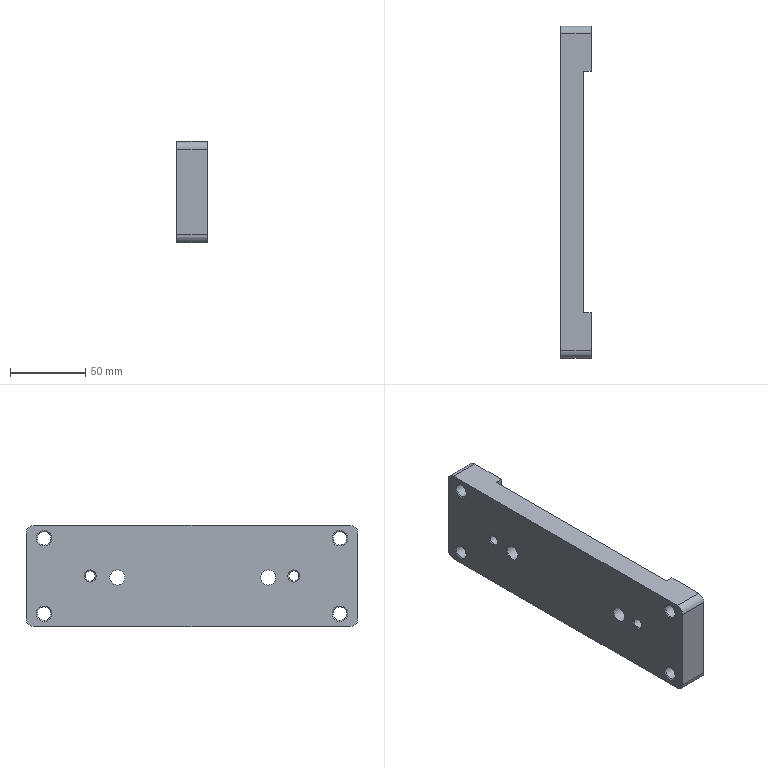Part | NX | features SIMPLE HOLE 8, DATUM_CSYS 7, SKETCH 6, EXTRUDE 3, HOLE PACKAGE 3, BLEND 2, SYMBOLIC_THREAD 2, LINKED_CURVE 1, LINKED_FACE 1 | 1 solid | 41 faces | box 20 x 220 x 67 mm | volume 225949 mm3 | cylinder 16 | plane 15 | cone 10 | commonest cylinder face diameters 10 x10 9 x4 6.8 x2
STEP:
#1=CARTESIAN_POINT('',(80.,80.,477.));
#2=VERTEX_POINT('',#1);
#3=CARTESIAN_POINT('',(80.,80.,410.));
#4=VERTEX_POINT('',#3);
#5=CARTESIAN_POINT('',(80.,80.,402.));
#6=DIRECTION('',(0.,0.,1.));
#7=VECTOR('',#6,1000.);
#8=LINE('',#5,#7);
#9=EDGE_CURVE('',#2,#4,#8,.F.);
#10=ORIENTED_EDGE('',*,*,#9,.F.);
#11=CARTESIAN_POINT('',(80.,-80.,477.));
#12=VERTEX_POINT('',#11);
#13=CARTESIAN_POINT('',(80.,80.,477.));
#14=DIRECTION('',(0.,-1.,0.));
#15=VECTOR('',#14,1000.);
#16=LINE('',#13,#15);
#17=EDGE_CURVE('',#2,#12,#16,.T.);
#18=ORIENTED_EDGE('',*,*,#17,.T.);
#19=CARTESIAN_POINT('',(80.,-80.,410.));
#20=VERTEX_POINT('',#19);
#21=CARTESIAN_POINT('',(80.,-80.,402.));
#22=DIRECTION('',(0.,0.,1.));
#23=VECTOR('',#22,1000.);
#24=LINE('',#21,#23);
#25=EDGE_CURVE('',#12,#20,#24,.F.);
#26=ORIENTED_EDGE('',*,*,#25,.T.);
#27=CARTESIAN_POINT('',(80.,-110.,410.));
#28=DIRECTION('',(0.,-1.,0.));
#29=VECTOR('',#28,1000.);
#30=LINE('',#27,#29);
#31=EDGE_CURVE('',#4,#20,#30,.T.);
#32=ORIENTED_EDGE('',*,*,#31,.F.);
#33=EDGE_LOOP('',(#10,#18,#26,#32));
#34=FACE_BOUND('',#33,.T.);
#35=CARTESIAN_POINT('',(80.,-67.5,446.9));
#36=VERTEX_POINT('',#35);
#37=CARTESIAN_POINT('',(80.,-67.5,443.5));
#38=DIRECTION('',(-1.,0.,0.));
#39=DIRECTION('',(0.,0.,1.));
#40=AXIS2_PLACEMENT_3D('',#37,#38,#39);
#41=CIRCLE('',#40,3.4);
#42=EDGE_CURVE('',#36,#36,#41,.F.);
#43=ORIENTED_EDGE('',*,*,#42,.F.);
#44=EDGE_LOOP('',(#43));
#45=FACE_BOUND('',#44,.T.);
#46=CARTESIAN_POINT('',(80.,67.5,446.9));
#47=VERTEX_POINT('',#46);
#48=CARTESIAN_POINT('',(80.,67.5,443.5));
#49=DIRECTION('',(-1.,0.,0.));
#50=DIRECTION('',(0.,0.,1.));
#51=AXIS2_PLACEMENT_3D('',#48,#49,#50);
#52=CIRCLE('',#51,3.4);
#53=EDGE_CURVE('',#47,#47,#52,.F.);
#54=ORIENTED_EDGE('',*,*,#53,.F.);
#55=EDGE_LOOP('',(#54));
#56=FACE_BOUND('',#55,.T.);
#57=CARTESIAN_POINT('',(80.,49.5,447.5));
#58=VERTEX_POINT('',#57);
#59=CARTESIAN_POINT('',(80.,49.5,442.5));
#60=DIRECTION('',(-1.,0.,0.));
#61=DIRECTION('',(0.,0.,1.));
#62=AXIS2_PLACEMENT_3D('',#59,#60,#61);
#63=CIRCLE('',#62,5.);
#64=EDGE_CURVE('',#58,#58,#63,.T.);
#65=ORIENTED_EDGE('',*,*,#64,.T.);
#66=EDGE_LOOP('',(#65));
#67=FACE_BOUND('',#66,.T.);
#68=CARTESIAN_POINT('',(80.,-50.5,447.5));
#69=VERTEX_POINT('',#68);
#70=CARTESIAN_POINT('',(80.,-50.5,442.5));
#71=DIRECTION('',(-1.,0.,0.));
#72=DIRECTION('',(0.,0.,1.));
#73=AXIS2_PLACEMENT_3D('',#70,#71,#72);
#74=CIRCLE('',#73,5.);
#75=EDGE_CURVE('',#69,#69,#74,.T.);
#76=ORIENTED_EDGE('',*,*,#75,.T.);
#77=EDGE_LOOP('',(#76));
#78=FACE_BOUND('',#77,.T.);
#79=CARTESIAN_POINT('',(80.,-30.5,456.));
#80=VERTEX_POINT('',#79);
#81=CARTESIAN_POINT('',(80.,-30.5,431.));
#82=VERTEX_POINT('',#81);
#83=CARTESIAN_POINT('',(80.,-30.5,461.));
#84=DIRECTION('',(0.,0.,-1.));
#85=VECTOR('',#84,1000.);
#86=LINE('',#83,#85);
#87=EDGE_CURVE('',#80,#82,#86,.T.);
#88=ORIENTED_EDGE('',*,*,#87,.F.);
#89=CARTESIAN_POINT('',(80.,-25.5,461.));
#90=VERTEX_POINT('',#89);
#91=CARTESIAN_POINT('',(80.,-25.5,456.));
#92=DIRECTION('',(-1.,0.,0.));
#93=DIRECTION('',(0.,0.,1.));
#94=AXIS2_PLACEMENT_3D('',#91,#92,#93);
#95=CIRCLE('',#94,5.);
#96=EDGE_CURVE('',#80,#90,#95,.T.);
#97=ORIENTED_EDGE('',*,*,#96,.T.);
#98=CARTESIAN_POINT('',(80.,24.5,461.));
#99=VERTEX_POINT('',#98);
#100=CARTESIAN_POINT('',(80.,29.5,461.));
#101=DIRECTION('',(0.,-1.,0.));
#102=VECTOR('',#101,1000.);
#103=LINE('',#100,#102);
#104=EDGE_CURVE('',#99,#90,#103,.T.);
#105=ORIENTED_EDGE('',*,*,#104,.F.);
#106=CARTESIAN_POINT('',(80.,29.5,456.));
#107=VERTEX_POINT('',#106);
#108=CARTESIAN_POINT('',(80.,24.5,456.));
#109=DIRECTION('',(-1.,0.,0.));
#110=DIRECTION('',(0.,0.,1.));
#111=AXIS2_PLACEMENT_3D('',#108,#109,#110);
#112=CIRCLE('',#111,5.);
#113=EDGE_CURVE('',#99,#107,#112,.T.);
#114=ORIENTED_EDGE('',*,*,#113,.T.);
#115=CARTESIAN_POINT('',(80.,29.5,431.));
#116=VERTEX_POINT('',#115);
#117=CARTESIAN_POINT('',(80.,29.5,426.));
#118=DIRECTION('',(0.,0.,1.));
#119=VECTOR('',#118,1000.);
#120=LINE('',#117,#119);
#121=EDGE_CURVE('',#116,#107,#120,.T.);
#122=ORIENTED_EDGE('',*,*,#121,.F.);
#123=CARTESIAN_POINT('',(80.,24.5,426.));
#124=VERTEX_POINT('',#123);
#125=CARTESIAN_POINT('',(80.,24.5,431.));
#126=DIRECTION('',(-1.,0.,0.));
#127=DIRECTION('',(0.,0.,1.));
#128=AXIS2_PLACEMENT_3D('',#125,#126,#127);
#129=CIRCLE('',#128,5.);
#130=EDGE_CURVE('',#116,#124,#129,.T.);
#131=ORIENTED_EDGE('',*,*,#130,.T.);
#132=CARTESIAN_POINT('',(80.,-25.5,426.));
#133=VERTEX_POINT('',#132);
#134=CARTESIAN_POINT('',(80.,-30.5,426.));
#135=DIRECTION('',(0.,1.,0.));
#136=VECTOR('',#135,1000.);
#137=LINE('',#134,#136);
#138=EDGE_CURVE('',#133,#124,#137,.T.);
#139=ORIENTED_EDGE('',*,*,#138,.F.);
#140=CARTESIAN_POINT('',(80.,-25.5,431.));
#141=DIRECTION('',(-1.,0.,0.));
#142=DIRECTION('',(0.,0.,1.));
#143=AXIS2_PLACEMENT_3D('',#140,#141,#142);
#144=CIRCLE('',#143,5.);
#145=EDGE_CURVE('',#133,#82,#144,.T.);
#146=ORIENTED_EDGE('',*,*,#145,.T.);
#147=EDGE_LOOP('',(#88,#97,#105,#114,#122,#131,#139,#146));
#148=FACE_BOUND('',#147,.T.);
#149=CARTESIAN_POINT('',(80.,80.,402.));
#150=DIRECTION('',(-1.,0.,0.));
#151=DIRECTION('',(0.,0.,1.));
#152=AXIS2_PLACEMENT_3D('',#149,#150,#151);
#153=PLANE('',#152);
#154=ADVANCED_FACE('',(#34,#45,#56,#67,#78,#148),#153,.F.);
#155=CARTESIAN_POINT('',(85.,105.,477.));
#156=VERTEX_POINT('',#155);
#157=CARTESIAN_POINT('',(85.,80.,477.));
#158=VERTEX_POINT('',#157);
#159=CARTESIAN_POINT('',(85.,110.,477.));
#160=DIRECTION('',(0.,-1.,0.));
#161=VECTOR('',#160,1000.);
#162=LINE('',#159,#161);
#163=EDGE_CURVE('',#156,#158,#162,.T.);
#164=ORIENTED_EDGE('',*,*,#163,.F.);
#165=CARTESIAN_POINT('',(65.,105.,477.));
#166=VERTEX_POINT('',#165);
#167=CARTESIAN_POINT('',(85.,105.,477.));
#168=DIRECTION('',(-1.,0.,0.));
#169=VECTOR('',#168,1000.);
#170=LINE('',#167,#169);
#171=EDGE_CURVE('',#156,#166,#170,.T.);
#172=ORIENTED_EDGE('',*,*,#171,.T.);
#173=CARTESIAN_POINT('',(65.,-105.,477.));
#174=VERTEX_POINT('',#173);
#175=CARTESIAN_POINT('',(65.,110.,477.));
#176=DIRECTION('',(0.,-1.,0.));
#177=VECTOR('',#176,1000.);
#178=LINE('',#175,#177);
#179=EDGE_CURVE('',#166,#174,#178,.T.);
#180=ORIENTED_EDGE('',*,*,#179,.T.);
#181=CARTESIAN_POINT('',(85.,-105.,477.));
#182=VERTEX_POINT('',#181);
#183=CARTESIAN_POINT('',(85.,-105.,477.));
#184=DIRECTION('',(-1.,0.,0.));
#185=VECTOR('',#184,1000.);
#186=LINE('',#183,#185);
#187=EDGE_CURVE('',#174,#182,#186,.F.);
#188=ORIENTED_EDGE('',*,*,#187,.T.);
#189=CARTESIAN_POINT('',(85.,-80.,477.));
#190=VERTEX_POINT('',#189);
#191=CARTESIAN_POINT('',(85.,110.,477.));
#192=DIRECTION('',(0.,-1.,0.));
#193=VECTOR('',#192,1000.);
#194=LINE('',#191,#193);
#195=EDGE_CURVE('',#190,#182,#194,.T.);
#196=ORIENTED_EDGE('',*,*,#195,.F.);
#197=CARTESIAN_POINT('',(80.,-80.,477.));
#198=DIRECTION('',(1.,0.,0.));
#199=VECTOR('',#198,1000.);
#200=LINE('',#197,#199);
#201=EDGE_CURVE('',#12,#190,#200,.T.);
#202=ORIENTED_EDGE('',*,*,#201,.F.);
#203=ORIENTED_EDGE('',*,*,#17,.F.);
#204=CARTESIAN_POINT('',(118.,80.,477.));
#205=DIRECTION('',(-1.,0.,0.));
#206=VECTOR('',#205,1000.);
#207=LINE('',#204,#206);
#208=EDGE_CURVE('',#158,#2,#207,.T.);
#209=ORIENTED_EDGE('',*,*,#208,.F.);
#210=EDGE_LOOP('',(#164,#172,#180,#188,#196,#202,#203,#209));
#211=FACE_BOUND('',#210,.T.);
#212=CARTESIAN_POINT('',(85.,110.,477.));
#213=DIRECTION('',(0.,0.,-1.));
#214=DIRECTION('',(0.,1.,0.));
#215=AXIS2_PLACEMENT_3D('',#212,#213,#214);
#216=PLANE('',#215);
#217=ADVANCED_FACE('',(#211),#216,.F.);
#218=CARTESIAN_POINT('',(85.,-98.,463.4));
#219=VERTEX_POINT('',#218);
#220=CARTESIAN_POINT('',(85.,-98.,468.5));
#221=DIRECTION('',(1.,0.,0.));
#222=DIRECTION('',(0.,0.,-1.));
#223=AXIS2_PLACEMENT_3D('',#220,#221,#222);
#224=CIRCLE('',#223,5.1);
#225=EDGE_CURVE('',#219,#219,#224,.F.);
#226=ORIENTED_EDGE('',*,*,#225,.T.);
#227=EDGE_LOOP('',(#226));
#228=FACE_BOUND('',#227,.T.);
#229=CARTESIAN_POINT('',(85.,-98.,413.4));
#230=VERTEX_POINT('',#229);
#231=CARTESIAN_POINT('',(85.,-98.,418.5));
#232=DIRECTION('',(1.,0.,0.));
#233=DIRECTION('',(0.,0.,-1.));
#234=AXIS2_PLACEMENT_3D('',#231,#232,#233);
#235=CIRCLE('',#234,5.1);
#236=EDGE_CURVE('',#230,#230,#235,.F.);
#237=ORIENTED_EDGE('',*,*,#236,.T.);
#238=EDGE_LOOP('',(#237));
#239=FACE_BOUND('',#238,.T.);
#240=CARTESIAN_POINT('',(85.,-110.,472.));
#241=VERTEX_POINT('',#240);
#242=CARTESIAN_POINT('',(85.,-110.,415.));
#243=VERTEX_POINT('',#242);
#244=CARTESIAN_POINT('',(85.,-110.,477.));
#245=DIRECTION('',(0.,0.,-1.));
#246=VECTOR('',#245,1000.);
#247=LINE('',#244,#246);
#248=EDGE_CURVE('',#241,#243,#247,.T.);
#249=ORIENTED_EDGE('',*,*,#248,.T.);
#250=CARTESIAN_POINT('',(85.,-105.,410.));
#251=VERTEX_POINT('',#250);
#252=CARTESIAN_POINT('',(85.,-105.,415.));
#253=DIRECTION('',(1.,0.,0.));
#254=DIRECTION('',(0.,0.,-1.));
#255=AXIS2_PLACEMENT_3D('',#252,#253,#254);
#256=CIRCLE('',#255,5.);
#257=EDGE_CURVE('',#243,#251,#256,.T.);
#258=ORIENTED_EDGE('',*,*,#257,.T.);
#259=CARTESIAN_POINT('',(85.,-80.,410.));
#260=VERTEX_POINT('',#259);
#261=CARTESIAN_POINT('',(85.,-110.,410.));
#262=DIRECTION('',(0.,1.,0.));
#263=VECTOR('',#262,1000.);
#264=LINE('',#261,#263);
#265=EDGE_CURVE('',#251,#260,#264,.T.);
#266=ORIENTED_EDGE('',*,*,#265,.T.);
#267=CARTESIAN_POINT('',(85.,-80.,0.));
#268=DIRECTION('',(0.,0.,-1.));
#269=VECTOR('',#268,1000.);
#270=LINE('',#267,#269);
#271=EDGE_CURVE('',#190,#260,#270,.T.);
#272=ORIENTED_EDGE('',*,*,#271,.F.);
#273=ORIENTED_EDGE('',*,*,#195,.T.);
#274=CARTESIAN_POINT('',(85.,-105.,472.));
#275=DIRECTION('',(1.,0.,0.));
#276=DIRECTION('',(0.,0.,-1.));
#277=AXIS2_PLACEMENT_3D('',#274,#275,#276);
#278=CIRCLE('',#277,5.);
#279=EDGE_CURVE('',#182,#241,#278,.T.);
#280=ORIENTED_EDGE('',*,*,#279,.T.);
#281=EDGE_LOOP('',(#249,#258,#266,#272,#273,#280));
#282=FACE_BOUND('',#281,.T.);
#283=CARTESIAN_POINT('',(85.,0.,0.));
#284=DIRECTION('',(1.,0.,0.));
#285=DIRECTION('',(0.,0.,-1.));
#286=AXIS2_PLACEMENT_3D('',#283,#284,#285);
#287=PLANE('',#286);
#288=ADVANCED_FACE('',(#228,#239,#282),#287,.T.);
#289=CARTESIAN_POINT('',(65.,-110.,472.));
#290=VERTEX_POINT('',#289);
#291=CARTESIAN_POINT('',(65.,-110.,415.));
#292=VERTEX_POINT('',#291);
#293=CARTESIAN_POINT('',(65.,-110.,477.));
#294=DIRECTION('',(0.,0.,-1.));
#295=VECTOR('',#294,1000.);
#296=LINE('',#293,#295);
#297=EDGE_CURVE('',#290,#292,#296,.T.);
#298=ORIENTED_EDGE('',*,*,#297,.T.);
#299=CARTESIAN_POINT('',(85.,-110.,415.));
#300=DIRECTION('',(-1.,0.,0.));
#301=VECTOR('',#300,1000.);
#302=LINE('',#299,#301);
#303=EDGE_CURVE('',#292,#243,#302,.F.);
#304=ORIENTED_EDGE('',*,*,#303,.T.);
#305=ORIENTED_EDGE('',*,*,#248,.F.);
#306=CARTESIAN_POINT('',(85.,-110.,472.));
#307=DIRECTION('',(-1.,0.,0.));
#308=VECTOR('',#307,1000.);
#309=LINE('',#306,#308);
#310=EDGE_CURVE('',#241,#290,#309,.T.);
#311=ORIENTED_EDGE('',*,*,#310,.T.);
#312=EDGE_LOOP('',(#298,#304,#305,#311));
#313=FACE_BOUND('',#312,.T.);
#314=CARTESIAN_POINT('',(85.,-110.,477.));
#315=DIRECTION('',(0.,1.,0.));
#316=DIRECTION('',(0.,0.,1.));
#317=AXIS2_PLACEMENT_3D('',#314,#315,#316);
#318=PLANE('',#317);
#319=ADVANCED_FACE('',(#313),#318,.F.);
#320=CARTESIAN_POINT('',(65.,-105.,410.));
#321=VERTEX_POINT('',#320);
#322=CARTESIAN_POINT('',(65.,105.,410.));
#323=VERTEX_POINT('',#322);
#324=CARTESIAN_POINT('',(65.,-110.,410.));
#325=DIRECTION('',(0.,1.,0.));
#326=VECTOR('',#325,1000.);
#327=LINE('',#324,#326);
#328=EDGE_CURVE('',#321,#323,#327,.T.);
#329=ORIENTED_EDGE('',*,*,#328,.T.);
#330=CARTESIAN_POINT('',(85.,105.,410.));
#331=VERTEX_POINT('',#330);
#332=CARTESIAN_POINT('',(85.,105.,410.));
#333=DIRECTION('',(-1.,0.,0.));
#334=VECTOR('',#333,1000.);
#335=LINE('',#332,#334);
#336=EDGE_CURVE('',#323,#331,#335,.F.);
#337=ORIENTED_EDGE('',*,*,#336,.T.);
#338=CARTESIAN_POINT('',(85.,80.,410.));
#339=VERTEX_POINT('',#338);
#340=CARTESIAN_POINT('',(85.,-110.,410.));
#341=DIRECTION('',(0.,1.,0.));
#342=VECTOR('',#341,1000.);
#343=LINE('',#340,#342);
#344=EDGE_CURVE('',#339,#331,#343,.T.);
#345=ORIENTED_EDGE('',*,*,#344,.F.);
#346=CARTESIAN_POINT('',(85.,80.,410.));
#347=DIRECTION('',(-1.,0.,0.));
#348=VECTOR('',#347,1000.);
#349=LINE('',#346,#348);
#350=EDGE_CURVE('',#339,#4,#349,.T.);
#351=ORIENTED_EDGE('',*,*,#350,.T.);
#352=ORIENTED_EDGE('',*,*,#31,.T.);
#353=CARTESIAN_POINT('',(85.,-80.,410.));
#354=DIRECTION('',(1.,0.,0.));
#355=VECTOR('',#354,1000.);
#356=LINE('',#353,#355);
#357=EDGE_CURVE('',#20,#260,#356,.T.);
#358=ORIENTED_EDGE('',*,*,#357,.T.);
#359=ORIENTED_EDGE('',*,*,#265,.F.);
#360=CARTESIAN_POINT('',(85.,-105.,410.));
#361=DIRECTION('',(-1.,0.,0.));
#362=VECTOR('',#361,1000.);
#363=LINE('',#360,#362);
#364=EDGE_CURVE('',#251,#321,#363,.T.);
#365=ORIENTED_EDGE('',*,*,#364,.T.);
#366=EDGE_LOOP('',(#329,#337,#345,#351,#352,#358,#359,#365));
#367=FACE_BOUND('',#366,.T.);
#368=CARTESIAN_POINT('',(85.,-110.,410.));
#369=DIRECTION('',(0.,0.,1.));
#370=DIRECTION('',(1.,0.,0.));
#371=AXIS2_PLACEMENT_3D('',#368,#369,#370);
#372=PLANE('',#371);
#373=ADVANCED_FACE('',(#367),#372,.F.);
#374=CARTESIAN_POINT('',(85.,110.,415.));
#375=VERTEX_POINT('',#374);
#376=CARTESIAN_POINT('',(85.,110.,472.));
#377=VERTEX_POINT('',#376);
#378=CARTESIAN_POINT('',(85.,110.,410.));
#379=DIRECTION('',(0.,0.,1.));
#380=VECTOR('',#379,1000.);
#381=LINE('',#378,#380);
#382=EDGE_CURVE('',#375,#377,#381,.T.);
#383=ORIENTED_EDGE('',*,*,#382,.F.);
#384=CARTESIAN_POINT('',(65.,110.,415.));
#385=VERTEX_POINT('',#384);
#386=CARTESIAN_POINT('',(85.,110.,415.));
#387=DIRECTION('',(-1.,0.,0.));
#388=VECTOR('',#387,1000.);
#389=LINE('',#386,#388);
#390=EDGE_CURVE('',#375,#385,#389,.T.);
#391=ORIENTED_EDGE('',*,*,#390,.T.);
#392=CARTESIAN_POINT('',(65.,110.,472.));
#393=VERTEX_POINT('',#392);
#394=CARTESIAN_POINT('',(65.,110.,410.));
#395=DIRECTION('',(0.,0.,1.));
#396=VECTOR('',#395,1000.);
#397=LINE('',#394,#396);
#398=EDGE_CURVE('',#385,#393,#397,.T.);
#399=ORIENTED_EDGE('',*,*,#398,.T.);
#400=CARTESIAN_POINT('',(85.,110.,472.));
#401=DIRECTION('',(-1.,0.,0.));
#402=VECTOR('',#401,1000.);
#403=LINE('',#400,#402);
#404=EDGE_CURVE('',#393,#377,#403,.F.);
#405=ORIENTED_EDGE('',*,*,#404,.T.);
#406=EDGE_LOOP('',(#383,#391,#399,#405));
#407=FACE_BOUND('',#406,.T.);
#408=CARTESIAN_POINT('',(85.,110.,410.));
#409=DIRECTION('',(0.,-1.,0.));
#410=DIRECTION('',(0.,0.,-1.));
#411=AXIS2_PLACEMENT_3D('',#408,#409,#410);
#412=PLANE('',#411);
#413=ADVANCED_FACE('',(#407),#412,.F.);
#414=CARTESIAN_POINT('',(85.,98.,463.4));
#415=VERTEX_POINT('',#414);
#416=CARTESIAN_POINT('',(85.,98.,468.5));
#417=DIRECTION('',(1.,0.,0.));
#418=DIRECTION('',(0.,0.,-1.));
#419=AXIS2_PLACEMENT_3D('',#416,#417,#418);
#420=CIRCLE('',#419,5.1);
#421=EDGE_CURVE('',#415,#415,#420,.F.);
#422=ORIENTED_EDGE('',*,*,#421,.T.);
#423=EDGE_LOOP('',(#422));
#424=FACE_BOUND('',#423,.T.);
#425=CARTESIAN_POINT('',(85.,98.,413.4));
#426=VERTEX_POINT('',#425);
#427=CARTESIAN_POINT('',(85.,98.,418.5));
#428=DIRECTION('',(1.,0.,0.));
#429=DIRECTION('',(0.,0.,-1.));
#430=AXIS2_PLACEMENT_3D('',#427,#428,#429);
#431=CIRCLE('',#430,5.1);
#432=EDGE_CURVE('',#426,#426,#431,.F.);
#433=ORIENTED_EDGE('',*,*,#432,.T.);
#434=EDGE_LOOP('',(#433));
#435=FACE_BOUND('',#434,.T.);
#436=ORIENTED_EDGE('',*,*,#344,.T.);
#437=CARTESIAN_POINT('',(85.,105.,415.));
#438=DIRECTION('',(1.,0.,0.));
#439=DIRECTION('',(0.,0.,-1.));
#440=AXIS2_PLACEMENT_3D('',#437,#438,#439);
#441=CIRCLE('',#440,5.);
#442=EDGE_CURVE('',#331,#375,#441,.T.);
#443=ORIENTED_EDGE('',*,*,#442,.T.);
#444=ORIENTED_EDGE('',*,*,#382,.T.);
#445=CARTESIAN_POINT('',(85.,105.,472.));
#446=DIRECTION('',(1.,0.,0.));
#447=DIRECTION('',(0.,0.,-1.));
#448=AXIS2_PLACEMENT_3D('',#445,#446,#447);
#449=CIRCLE('',#448,5.);
#450=EDGE_CURVE('',#377,#156,#449,.T.);
#451=ORIENTED_EDGE('',*,*,#450,.T.);
#452=ORIENTED_EDGE('',*,*,#163,.T.);
#453=CARTESIAN_POINT('',(85.,80.,0.));
#454=DIRECTION('',(0.,0.,1.));
#455=VECTOR('',#454,1000.);
#456=LINE('',#453,#455);
#457=EDGE_CURVE('',#339,#158,#456,.T.);
#458=ORIENTED_EDGE('',*,*,#457,.F.);
#459=EDGE_LOOP('',(#436,#443,#444,#451,#452,#458));
#460=FACE_BOUND('',#459,.T.);
#461=CARTESIAN_POINT('',(85.,0.,0.));
#462=DIRECTION('',(1.,0.,0.));
#463=DIRECTION('',(0.,0.,-1.));
#464=AXIS2_PLACEMENT_3D('',#461,#462,#463);
#465=PLANE('',#464);
#466=ADVANCED_FACE('',(#424,#435,#460),#465,.T.);
#467=CARTESIAN_POINT('',(65.,98.,463.4));
#468=VERTEX_POINT('',#467);
#469=CARTESIAN_POINT('',(65.,98.,468.5));
#470=DIRECTION('',(1.,0.,0.));
#471=DIRECTION('',(0.,0.,-1.));
#472=AXIS2_PLACEMENT_3D('',#469,#470,#471);
#473=CIRCLE('',#472,5.1);
#474=EDGE_CURVE('',#468,#468,#473,.T.);
#475=ORIENTED_EDGE('',*,*,#474,.T.);
#476=EDGE_LOOP('',(#475));
#477=FACE_BOUND('',#476,.T.);
#478=CARTESIAN_POINT('',(65.,98.,413.4));
#479=VERTEX_POINT('',#478);
#480=CARTESIAN_POINT('',(65.,98.,418.5));
#481=DIRECTION('',(1.,0.,0.));
#482=DIRECTION('',(0.,0.,-1.));
#483=AXIS2_PLACEMENT_3D('',#480,#481,#482);
#484=CIRCLE('',#483,5.1);
#485=EDGE_CURVE('',#479,#479,#484,.T.);
#486=ORIENTED_EDGE('',*,*,#485,.T.);
#487=EDGE_LOOP('',(#486));
#488=FACE_BOUND('',#487,.T.);
#489=CARTESIAN_POINT('',(65.,-98.,463.4));
#490=VERTEX_POINT('',#489);
#491=CARTESIAN_POINT('',(65.,-98.,468.5));
#492=DIRECTION('',(1.,0.,0.));
#493=DIRECTION('',(0.,0.,-1.));
#494=AXIS2_PLACEMENT_3D('',#491,#492,#493);
#495=CIRCLE('',#494,5.1);
#496=EDGE_CURVE('',#490,#490,#495,.T.);
#497=ORIENTED_EDGE('',*,*,#496,.T.);
#498=EDGE_LOOP('',(#497));
#499=FACE_BOUND('',#498,.T.);
#500=CARTESIAN_POINT('',(65.,-98.,413.4));
#501=VERTEX_POINT('',#500);
#502=CARTESIAN_POINT('',(65.,-98.,418.5));
#503=DIRECTION('',(1.,0.,0.));
#504=DIRECTION('',(0.,0.,-1.));
#505=AXIS2_PLACEMENT_3D('',#502,#503,#504);
#506=CIRCLE('',#505,5.1);
#507=EDGE_CURVE('',#501,#501,#506,.T.);
#508=ORIENTED_EDGE('',*,*,#507,.T.);
#509=EDGE_LOOP('',(#508));
#510=FACE_BOUND('',#509,.T.);
#511=CARTESIAN_POINT('',(65.,-50.5,437.5));
#512=VERTEX_POINT('',#511);
#513=CARTESIAN_POINT('',(65.,-50.5,442.5));
#514=DIRECTION('',(1.,0.,0.));
#515=DIRECTION('',(0.,0.,-1.));
#516=AXIS2_PLACEMENT_3D('',#513,#514,#515);
#517=CIRCLE('',#516,5.);
#518=EDGE_CURVE('',#512,#512,#517,.T.);
#519=ORIENTED_EDGE('',*,*,#518,.T.);
#520=EDGE_LOOP('',(#519));
#521=FACE_BOUND('',#520,.T.);
#522=CARTESIAN_POINT('',(65.,49.5,437.5));
#523=VERTEX_POINT('',#522);
#524=CARTESIAN_POINT('',(65.,49.5,442.5));
#525=DIRECTION('',(1.,0.,0.));
#526=DIRECTION('',(0.,0.,-1.));
#527=AXIS2_PLACEMENT_3D('',#524,#525,#526);
#528=CIRCLE('',#527,5.);
#529=EDGE_CURVE('',#523,#523,#528,.T.);
#530=ORIENTED_EDGE('',*,*,#529,.T.);
#531=EDGE_LOOP('',(#530));
#532=FACE_BOUND('',#531,.T.);
#533=CARTESIAN_POINT('',(65.,67.5,439.5));
#534=VERTEX_POINT('',#533);
#535=CARTESIAN_POINT('',(65.,67.5,443.5));
#536=DIRECTION('',(1.,0.,0.));
#537=DIRECTION('',(0.,0.,-1.));
#538=AXIS2_PLACEMENT_3D('',#535,#536,#537);
#539=CIRCLE('',#538,4.);
#540=EDGE_CURVE('',#534,#534,#539,.T.);
#541=ORIENTED_EDGE('',*,*,#540,.T.);
#542=EDGE_LOOP('',(#541));
#543=FACE_BOUND('',#542,.T.);
#544=CARTESIAN_POINT('',(65.,-67.5,439.5));
#545=VERTEX_POINT('',#544);
#546=CARTESIAN_POINT('',(65.,-67.5,443.5));
#547=DIRECTION('',(1.,0.,0.));
#548=DIRECTION('',(0.,0.,-1.));
#549=AXIS2_PLACEMENT_3D('',#546,#547,#548);
#550=CIRCLE('',#549,4.);
#551=EDGE_CURVE('',#545,#545,#550,.T.);
#552=ORIENTED_EDGE('',*,*,#551,.T.);
#553=EDGE_LOOP('',(#552));
#554=FACE_BOUND('',#553,.T.);
#555=ORIENTED_EDGE('',*,*,#398,.F.);
#556=CARTESIAN_POINT('',(65.,105.,415.));
#557=DIRECTION('',(1.,0.,0.));
#558=DIRECTION('',(0.,0.,-1.));
#559=AXIS2_PLACEMENT_3D('',#556,#557,#558);
#560=CIRCLE('',#559,5.);
#561=EDGE_CURVE('',#385,#323,#560,.F.);
#562=ORIENTED_EDGE('',*,*,#561,.T.);
#563=ORIENTED_EDGE('',*,*,#328,.F.);
#564=CARTESIAN_POINT('',(65.,-105.,415.));
#565=DIRECTION('',(1.,0.,0.));
#566=DIRECTION('',(0.,0.,-1.));
#567=AXIS2_PLACEMENT_3D('',#564,#565,#566);
#568=CIRCLE('',#567,5.);
#569=EDGE_CURVE('',#321,#292,#568,.F.);
#570=ORIENTED_EDGE('',*,*,#569,.T.);
#571=ORIENTED_EDGE('',*,*,#297,.F.);
#572=CARTESIAN_POINT('',(65.,-105.,472.));
#573=DIRECTION('',(1.,0.,0.));
#574=DIRECTION('',(0.,0.,-1.));
#575=AXIS2_PLACEMENT_3D('',#572,#573,#574);
#576=CIRCLE('',#575,5.);
#577=EDGE_CURVE('',#290,#174,#576,.F.);
#578=ORIENTED_EDGE('',*,*,#577,.T.);
#579=ORIENTED_EDGE('',*,*,#179,.F.);
#580=CARTESIAN_POINT('',(65.,105.,472.));
#581=DIRECTION('',(1.,0.,0.));
#582=DIRECTION('',(0.,0.,-1.));
#583=AXIS2_PLACEMENT_3D('',#580,#581,#582);
#584=CIRCLE('',#583,5.);
#585=EDGE_CURVE('',#166,#393,#584,.F.);
#586=ORIENTED_EDGE('',*,*,#585,.T.);
#587=EDGE_LOOP('',(#555,#562,#563,#570,#571,#578,#579,#586));
#588=FACE_BOUND('',#587,.T.);
#589=CARTESIAN_POINT('',(65.,0.,0.));
#590=DIRECTION('',(1.,0.,0.));
#591=DIRECTION('',(0.,0.,-1.));
#592=AXIS2_PLACEMENT_3D('',#589,#590,#591);
#593=PLANE('',#592);
#594=ADVANCED_FACE('',(#477,#488,#499,#510,#521,#532,#543,#554,#588),#593,.F.);
#595=ORIENTED_EDGE('',*,*,#42,.T.);
#596=EDGE_LOOP('',(#595));
#597=FACE_BOUND('',#596,.T.);
#598=CARTESIAN_POINT('',(65.6,-67.5,440.1));
#599=VERTEX_POINT('',#598);
#600=CARTESIAN_POINT('',(65.6,-67.5,443.5));
#601=DIRECTION('',(1.,0.,0.));
#602=DIRECTION('',(0.,0.,-1.));
#603=AXIS2_PLACEMENT_3D('',#600,#601,#602);
#604=CIRCLE('',#603,3.4);
#605=EDGE_CURVE('',#599,#599,#604,.F.);
#606=ORIENTED_EDGE('',*,*,#605,.T.);
#607=EDGE_LOOP('',(#606));
#608=FACE_BOUND('',#607,.T.);
#609=CARTESIAN_POINT('',(65.,-67.5,443.5));
#610=DIRECTION('',(1.,0.,0.));
#611=DIRECTION('',(0.,0.,-1.));
#612=AXIS2_PLACEMENT_3D('',#609,#610,#611);
#613=CYLINDRICAL_SURFACE('',#612,3.4);
#614=ADVANCED_FACE('',(#597,#608),#613,.F.);
#615=ORIENTED_EDGE('',*,*,#605,.F.);
#616=EDGE_LOOP('',(#615));
#617=FACE_BOUND('',#616,.T.);
#618=ORIENTED_EDGE('',*,*,#551,.F.);
#619=EDGE_LOOP('',(#618));
#620=FACE_BOUND('',#619,.T.);
#621=CARTESIAN_POINT('',(65.,-67.5,443.5));
#622=DIRECTION('',(-1.,0.,0.));
#623=DIRECTION('',(0.,0.,1.));
#624=AXIS2_PLACEMENT_3D('',#621,#622,#623);
#625=CONICAL_SURFACE('',#624,4.,0.7854);
#626=ADVANCED_FACE('',(#617,#620),#625,.F.);
#627=ORIENTED_EDGE('',*,*,#53,.T.);
#628=EDGE_LOOP('',(#627));
#629=FACE_BOUND('',#628,.T.);
#630=CARTESIAN_POINT('',(65.6,67.5,440.1));
#631=VERTEX_POINT('',#630);
#632=CARTESIAN_POINT('',(65.6,67.5,443.5));
#633=DIRECTION('',(1.,0.,0.));
#634=DIRECTION('',(0.,0.,-1.));
#635=AXIS2_PLACEMENT_3D('',#632,#633,#634);
#636=CIRCLE('',#635,3.4);
#637=EDGE_CURVE('',#631,#631,#636,.F.);
#638=ORIENTED_EDGE('',*,*,#637,.T.);
#639=EDGE_LOOP('',(#638));
#640=FACE_BOUND('',#639,.T.);
#641=CARTESIAN_POINT('',(65.,67.5,443.5));
#642=DIRECTION('',(1.,0.,0.));
#643=DIRECTION('',(0.,0.,-1.));
#644=AXIS2_PLACEMENT_3D('',#641,#642,#643);
#645=CYLINDRICAL_SURFACE('',#644,3.4);
#646=ADVANCED_FACE('',(#629,#640),#645,.F.);
#647=ORIENTED_EDGE('',*,*,#637,.F.);
#648=EDGE_LOOP('',(#647));
#649=FACE_BOUND('',#648,.T.);
#650=ORIENTED_EDGE('',*,*,#540,.F.);
#651=EDGE_LOOP('',(#650));
#652=FACE_BOUND('',#651,.T.);
#653=CARTESIAN_POINT('',(65.,67.5,443.5));
#654=DIRECTION('',(-1.,0.,0.));
#655=DIRECTION('',(0.,0.,1.));
#656=AXIS2_PLACEMENT_3D('',#653,#654,#655);
#657=CONICAL_SURFACE('',#656,4.,0.7854);
#658=ADVANCED_FACE('',(#649,#652),#657,.F.);
#659=ORIENTED_EDGE('',*,*,#25,.F.);
#660=ORIENTED_EDGE('',*,*,#201,.T.);
#661=ORIENTED_EDGE('',*,*,#271,.T.);
#662=ORIENTED_EDGE('',*,*,#357,.F.);
#663=EDGE_LOOP('',(#659,#660,#661,#662));
#664=FACE_BOUND('',#663,.T.);
#665=CARTESIAN_POINT('',(80.,-80.,402.));
#666=DIRECTION('',(0.,-1.,0.));
#667=DIRECTION('',(0.,0.,-1.));
#668=AXIS2_PLACEMENT_3D('',#665,#666,#667);
#669=PLANE('',#668);
#670=ADVANCED_FACE('',(#664),#669,.F.);
#671=ORIENTED_EDGE('',*,*,#457,.T.);
#672=ORIENTED_EDGE('',*,*,#208,.T.);
#673=ORIENTED_EDGE('',*,*,#9,.T.);
#674=ORIENTED_EDGE('',*,*,#350,.F.);
#675=EDGE_LOOP('',(#671,#672,#673,#674));
#676=FACE_BOUND('',#675,.T.);
#677=CARTESIAN_POINT('',(118.,80.,402.));
#678=DIRECTION('',(0.,1.,0.));
#679=DIRECTION('',(0.,0.,1.));
#680=AXIS2_PLACEMENT_3D('',#677,#678,#679);
#681=PLANE('',#680);
#682=ADVANCED_FACE('',(#676),#681,.F.);
#683=ORIENTED_EDGE('',*,*,#442,.F.);
#684=ORIENTED_EDGE('',*,*,#336,.F.);
#685=ORIENTED_EDGE('',*,*,#561,.F.);
#686=ORIENTED_EDGE('',*,*,#390,.F.);
#687=EDGE_LOOP('',(#683,#684,#685,#686));
#688=FACE_BOUND('',#687,.T.);
#689=CARTESIAN_POINT('',(85.,105.,415.));
#690=DIRECTION('',(-1.,0.,0.));
#691=DIRECTION('',(0.,0.,1.));
#692=AXIS2_PLACEMENT_3D('',#689,#690,#691);
#693=CYLINDRICAL_SURFACE('',#692,5.);
#694=ADVANCED_FACE('',(#688),#693,.T.);
#695=ORIENTED_EDGE('',*,*,#450,.F.);
#696=ORIENTED_EDGE('',*,*,#404,.F.);
#697=ORIENTED_EDGE('',*,*,#585,.F.);
#698=ORIENTED_EDGE('',*,*,#171,.F.);
#699=EDGE_LOOP('',(#695,#696,#697,#698));
#700=FACE_BOUND('',#699,.T.);
#701=CARTESIAN_POINT('',(85.,105.,472.));
#702=DIRECTION('',(-1.,0.,0.));
#703=DIRECTION('',(0.,0.,1.));
#704=AXIS2_PLACEMENT_3D('',#701,#702,#703);
#705=CYLINDRICAL_SURFACE('',#704,5.);
#706=ADVANCED_FACE('',(#700),#705,.T.);
#707=ORIENTED_EDGE('',*,*,#257,.F.);
#708=ORIENTED_EDGE('',*,*,#303,.F.);
#709=ORIENTED_EDGE('',*,*,#569,.F.);
#710=ORIENTED_EDGE('',*,*,#364,.F.);
#711=EDGE_LOOP('',(#707,#708,#709,#710));
#712=FACE_BOUND('',#711,.T.);
#713=CARTESIAN_POINT('',(85.,-105.,415.));
#714=DIRECTION('',(-1.,0.,0.));
#715=DIRECTION('',(0.,0.,1.));
#716=AXIS2_PLACEMENT_3D('',#713,#714,#715);
#717=CYLINDRICAL_SURFACE('',#716,5.);
#718=ADVANCED_FACE('',(#712),#717,.T.);
#719=ORIENTED_EDGE('',*,*,#279,.F.);
#720=ORIENTED_EDGE('',*,*,#187,.F.);
#721=ORIENTED_EDGE('',*,*,#577,.F.);
#722=ORIENTED_EDGE('',*,*,#310,.F.);
#723=EDGE_LOOP('',(#719,#720,#721,#722));
#724=FACE_BOUND('',#723,.T.);
#725=CARTESIAN_POINT('',(85.,-105.,472.));
#726=DIRECTION('',(-1.,0.,0.));
#727=DIRECTION('',(0.,0.,1.));
#728=AXIS2_PLACEMENT_3D('',#725,#726,#727);
#729=CYLINDRICAL_SURFACE('',#728,5.);
#730=ADVANCED_FACE('',(#724),#729,.T.);
#731=ORIENTED_EDGE('',*,*,#529,.F.);
#732=EDGE_LOOP('',(#731));
#733=FACE_BOUND('',#732,.T.);
#734=ORIENTED_EDGE('',*,*,#64,.F.);
#735=EDGE_LOOP('',(#734));
#736=FACE_BOUND('',#735,.T.);
#737=CARTESIAN_POINT('',(65.,49.5,442.5));
#738=DIRECTION('',(1.,0.,0.));
#739=DIRECTION('',(0.,0.,-1.));
#740=AXIS2_PLACEMENT_3D('',#737,#738,#739);
#741=CYLINDRICAL_SURFACE('',#740,5.);
#742=ADVANCED_FACE('',(#733,#736),#741,.F.);
#743=ORIENTED_EDGE('',*,*,#518,.F.);
#744=EDGE_LOOP('',(#743));
#745=FACE_BOUND('',#744,.T.);
#746=ORIENTED_EDGE('',*,*,#75,.F.);
#747=EDGE_LOOP('',(#746));
#748=FACE_BOUND('',#747,.T.);
#749=CARTESIAN_POINT('',(65.,-50.5,442.5));
#750=DIRECTION('',(1.,0.,0.));
#751=DIRECTION('',(0.,0.,-1.));
#752=AXIS2_PLACEMENT_3D('',#749,#750,#751);
#753=CYLINDRICAL_SURFACE('',#752,5.);
#754=ADVANCED_FACE('',(#745,#748),#753,.F.);
#755=CARTESIAN_POINT('',(84.4,-98.,414.));
#756=VERTEX_POINT('',#755);
#757=CARTESIAN_POINT('',(84.4,-98.,418.5));
#758=DIRECTION('',(1.,0.,0.));
#759=DIRECTION('',(0.,0.,-1.));
#760=AXIS2_PLACEMENT_3D('',#757,#758,#759);
#761=CIRCLE('',#760,4.5);
#762=EDGE_CURVE('',#756,#756,#761,.T.);
#763=ORIENTED_EDGE('',*,*,#762,.T.);
#764=EDGE_LOOP('',(#763));
#765=FACE_BOUND('',#764,.T.);
#766=CARTESIAN_POINT('',(65.6,-98.,414.));
#767=VERTEX_POINT('',#766);
#768=CARTESIAN_POINT('',(65.6,-98.,418.5));
#769=DIRECTION('',(1.,0.,0.));
#770=DIRECTION('',(0.,0.,-1.));
#771=AXIS2_PLACEMENT_3D('',#768,#769,#770);
#772=CIRCLE('',#771,4.5);
#773=EDGE_CURVE('',#767,#767,#772,.F.);
#774=ORIENTED_EDGE('',*,*,#773,.T.);
#775=EDGE_LOOP('',(#774));
#776=FACE_BOUND('',#775,.T.);
#777=CARTESIAN_POINT('',(65.,-98.,418.5));
#778=DIRECTION('',(1.,0.,0.));
#779=DIRECTION('',(0.,0.,-1.));
#780=AXIS2_PLACEMENT_3D('',#777,#778,#779);
#781=CYLINDRICAL_SURFACE('',#780,4.5);
#782=ADVANCED_FACE('',(#765,#776),#781,.F.);
#783=ORIENTED_EDGE('',*,*,#773,.F.);
#784=EDGE_LOOP('',(#783));
#785=FACE_BOUND('',#784,.T.);
#786=ORIENTED_EDGE('',*,*,#507,.F.);
#787=EDGE_LOOP('',(#786));
#788=FACE_BOUND('',#787,.T.);
#789=CARTESIAN_POINT('',(65.,-98.,418.5));
#790=DIRECTION('',(-1.,0.,0.));
#791=DIRECTION('',(0.,0.,1.));
#792=AXIS2_PLACEMENT_3D('',#789,#790,#791);
#793=CONICAL_SURFACE('',#792,5.1,0.7854);
#794=ADVANCED_FACE('',(#785,#788),#793,.F.);
#795=ORIENTED_EDGE('',*,*,#236,.F.);
#796=EDGE_LOOP('',(#795));
#797=FACE_BOUND('',#796,.T.);
#798=ORIENTED_EDGE('',*,*,#762,.F.);
#799=EDGE_LOOP('',(#798));
#800=FACE_BOUND('',#799,.T.);
#801=CARTESIAN_POINT('',(84.4,-98.,418.5));
#802=DIRECTION('',(1.,0.,0.));
#803=DIRECTION('',(0.,0.,-1.));
#804=AXIS2_PLACEMENT_3D('',#801,#802,#803);
#805=CONICAL_SURFACE('',#804,4.5,0.7854);
#806=ADVANCED_FACE('',(#797,#800),#805,.F.);
#807=CARTESIAN_POINT('',(84.4,-98.,464.));
#808=VERTEX_POINT('',#807);
#809=CARTESIAN_POINT('',(84.4,-98.,468.5));
#810=DIRECTION('',(1.,0.,0.));
#811=DIRECTION('',(0.,0.,-1.));
#812=AXIS2_PLACEMENT_3D('',#809,#810,#811);
#813=CIRCLE('',#812,4.5);
#814=EDGE_CURVE('',#808,#808,#813,.T.);
#815=ORIENTED_EDGE('',*,*,#814,.T.);
#816=EDGE_LOOP('',(#815));
#817=FACE_BOUND('',#816,.T.);
#818=CARTESIAN_POINT('',(65.6,-98.,464.));
#819=VERTEX_POINT('',#818);
#820=CARTESIAN_POINT('',(65.6,-98.,468.5));
#821=DIRECTION('',(1.,0.,0.));
#822=DIRECTION('',(0.,0.,-1.));
#823=AXIS2_PLACEMENT_3D('',#820,#821,#822);
#824=CIRCLE('',#823,4.5);
#825=EDGE_CURVE('',#819,#819,#824,.F.);
#826=ORIENTED_EDGE('',*,*,#825,.T.);
#827=EDGE_LOOP('',(#826));
#828=FACE_BOUND('',#827,.T.);
#829=CARTESIAN_POINT('',(65.,-98.,468.5));
#830=DIRECTION('',(1.,0.,0.));
#831=DIRECTION('',(0.,0.,-1.));
#832=AXIS2_PLACEMENT_3D('',#829,#830,#831);
#833=CYLINDRICAL_SURFACE('',#832,4.5);
#834=ADVANCED_FACE('',(#817,#828),#833,.F.);
#835=ORIENTED_EDGE('',*,*,#825,.F.);
#836=EDGE_LOOP('',(#835));
#837=FACE_BOUND('',#836,.T.);
#838=ORIENTED_EDGE('',*,*,#496,.F.);
#839=EDGE_LOOP('',(#838));
#840=FACE_BOUND('',#839,.T.);
#841=CARTESIAN_POINT('',(65.,-98.,468.5));
#842=DIRECTION('',(-1.,0.,0.));
#843=DIRECTION('',(0.,0.,1.));
#844=AXIS2_PLACEMENT_3D('',#841,#842,#843);
#845=CONICAL_SURFACE('',#844,5.1,0.7854);
#846=ADVANCED_FACE('',(#837,#840),#845,.F.);
#847=ORIENTED_EDGE('',*,*,#225,.F.);
#848=EDGE_LOOP('',(#847));
#849=FACE_BOUND('',#848,.T.);
#850=ORIENTED_EDGE('',*,*,#814,.F.);
#851=EDGE_LOOP('',(#850));
#852=FACE_BOUND('',#851,.T.);
#853=CARTESIAN_POINT('',(84.4,-98.,468.5));
#854=DIRECTION('',(1.,0.,0.));
#855=DIRECTION('',(0.,0.,-1.));
#856=AXIS2_PLACEMENT_3D('',#853,#854,#855);
#857=CONICAL_SURFACE('',#856,4.5,0.7854);
#858=ADVANCED_FACE('',(#849,#852),#857,.F.);
#859=CARTESIAN_POINT('',(84.4,98.,414.));
#860=VERTEX_POINT('',#859);
#861=CARTESIAN_POINT('',(84.4,98.,418.5));
#862=DIRECTION('',(1.,0.,0.));
#863=DIRECTION('',(0.,0.,-1.));
#864=AXIS2_PLACEMENT_3D('',#861,#862,#863);
#865=CIRCLE('',#864,4.5);
#866=EDGE_CURVE('',#860,#860,#865,.T.);
#867=ORIENTED_EDGE('',*,*,#866,.T.);
#868=EDGE_LOOP('',(#867));
#869=FACE_BOUND('',#868,.T.);
#870=CARTESIAN_POINT('',(65.6,98.,414.));
#871=VERTEX_POINT('',#870);
#872=CARTESIAN_POINT('',(65.6,98.,418.5));
#873=DIRECTION('',(1.,0.,0.));
#874=DIRECTION('',(0.,0.,-1.));
#875=AXIS2_PLACEMENT_3D('',#872,#873,#874);
#876=CIRCLE('',#875,4.5);
#877=EDGE_CURVE('',#871,#871,#876,.F.);
#878=ORIENTED_EDGE('',*,*,#877,.T.);
#879=EDGE_LOOP('',(#878));
#880=FACE_BOUND('',#879,.T.);
#881=CARTESIAN_POINT('',(65.,98.,418.5));
#882=DIRECTION('',(1.,0.,0.));
#883=DIRECTION('',(0.,0.,-1.));
#884=AXIS2_PLACEMENT_3D('',#881,#882,#883);
#885=CYLINDRICAL_SURFACE('',#884,4.5);
#886=ADVANCED_FACE('',(#869,#880),#885,.F.);
#887=ORIENTED_EDGE('',*,*,#877,.F.);
#888=EDGE_LOOP('',(#887));
#889=FACE_BOUND('',#888,.T.);
#890=ORIENTED_EDGE('',*,*,#485,.F.);
#891=EDGE_LOOP('',(#890));
#892=FACE_BOUND('',#891,.T.);
#893=CARTESIAN_POINT('',(65.,98.,418.5));
#894=DIRECTION('',(-1.,0.,0.));
#895=DIRECTION('',(0.,0.,1.));
#896=AXIS2_PLACEMENT_3D('',#893,#894,#895);
#897=CONICAL_SURFACE('',#896,5.1,0.7854);
#898=ADVANCED_FACE('',(#889,#892),#897,.F.);
#899=ORIENTED_EDGE('',*,*,#432,.F.);
#900=EDGE_LOOP('',(#899));
#901=FACE_BOUND('',#900,.T.);
#902=ORIENTED_EDGE('',*,*,#866,.F.);
#903=EDGE_LOOP('',(#902));
#904=FACE_BOUND('',#903,.T.);
#905=CARTESIAN_POINT('',(84.4,98.,418.5));
#906=DIRECTION('',(1.,0.,0.));
#907=DIRECTION('',(0.,0.,-1.));
#908=AXIS2_PLACEMENT_3D('',#905,#906,#907);
#909=CONICAL_SURFACE('',#908,4.5,0.7854);
#910=ADVANCED_FACE('',(#901,#904),#909,.F.);
#911=CARTESIAN_POINT('',(84.4,98.,464.));
#912=VERTEX_POINT('',#911);
#913=CARTESIAN_POINT('',(84.4,98.,468.5));
#914=DIRECTION('',(1.,0.,0.));
#915=DIRECTION('',(0.,0.,-1.));
#916=AXIS2_PLACEMENT_3D('',#913,#914,#915);
#917=CIRCLE('',#916,4.5);
#918=EDGE_CURVE('',#912,#912,#917,.T.);
#919=ORIENTED_EDGE('',*,*,#918,.T.);
#920=EDGE_LOOP('',(#919));
#921=FACE_BOUND('',#920,.T.);
#922=CARTESIAN_POINT('',(65.6,98.,464.));
#923=VERTEX_POINT('',#922);
#924=CARTESIAN_POINT('',(65.6,98.,468.5));
#925=DIRECTION('',(1.,0.,0.));
#926=DIRECTION('',(0.,0.,-1.));
#927=AXIS2_PLACEMENT_3D('',#924,#925,#926);
#928=CIRCLE('',#927,4.5);
#929=EDGE_CURVE('',#923,#923,#928,.F.);
#930=ORIENTED_EDGE('',*,*,#929,.T.);
#931=EDGE_LOOP('',(#930));
#932=FACE_BOUND('',#931,.T.);
#933=CARTESIAN_POINT('',(65.,98.,468.5));
#934=DIRECTION('',(1.,0.,0.));
#935=DIRECTION('',(0.,0.,-1.));
#936=AXIS2_PLACEMENT_3D('',#933,#934,#935);
#937=CYLINDRICAL_SURFACE('',#936,4.5);
#938=ADVANCED_FACE('',(#921,#932),#937,.F.);
#939=ORIENTED_EDGE('',*,*,#929,.F.);
#940=EDGE_LOOP('',(#939));
#941=FACE_BOUND('',#940,.T.);
#942=ORIENTED_EDGE('',*,*,#474,.F.);
#943=EDGE_LOOP('',(#942));
#944=FACE_BOUND('',#943,.T.);
#945=CARTESIAN_POINT('',(65.,98.,468.5));
#946=DIRECTION('',(-1.,0.,0.));
#947=DIRECTION('',(0.,0.,1.));
#948=AXIS2_PLACEMENT_3D('',#945,#946,#947);
#949=CONICAL_SURFACE('',#948,5.1,0.7854);
#950=ADVANCED_FACE('',(#941,#944),#949,.F.);
#951=ORIENTED_EDGE('',*,*,#421,.F.);
#952=EDGE_LOOP('',(#951));
#953=FACE_BOUND('',#952,.T.);
#954=ORIENTED_EDGE('',*,*,#918,.F.);
#955=EDGE_LOOP('',(#954));
#956=FACE_BOUND('',#955,.T.);
#957=CARTESIAN_POINT('',(84.4,98.,468.5));
#958=DIRECTION('',(1.,0.,0.));
#959=DIRECTION('',(0.,0.,-1.));
#960=AXIS2_PLACEMENT_3D('',#957,#958,#959);
#961=CONICAL_SURFACE('',#960,4.5,0.7854);
#962=ADVANCED_FACE('',(#953,#956),#961,.F.);
#963=ORIENTED_EDGE('',*,*,#87,.T.);
#964=CARTESIAN_POINT('',(77.,-30.5,431.));
#965=VERTEX_POINT('',#964);
#966=CARTESIAN_POINT('',(77.,-30.5,431.));
#967=DIRECTION('',(-1.,0.,0.));
#968=VECTOR('',#967,1000.);
#969=LINE('',#966,#968);
#970=EDGE_CURVE('',#82,#965,#969,.T.);
#971=ORIENTED_EDGE('',*,*,#970,.T.);
#972=CARTESIAN_POINT('',(77.,-30.5,456.));
#973=VERTEX_POINT('',#972);
#974=CARTESIAN_POINT('',(77.,-30.5,461.));
#975=DIRECTION('',(0.,0.,-1.));
#976=VECTOR('',#975,1000.);
#977=LINE('',#974,#976);
#978=EDGE_CURVE('',#965,#973,#977,.F.);
#979=ORIENTED_EDGE('',*,*,#978,.T.);
#980=CARTESIAN_POINT('',(80.,-30.5,456.));
#981=DIRECTION('',(-1.,0.,0.));
#982=VECTOR('',#981,1000.);
#983=LINE('',#980,#982);
#984=EDGE_CURVE('',#973,#80,#983,.F.);
#985=ORIENTED_EDGE('',*,*,#984,.T.);
#986=EDGE_LOOP('',(#963,#971,#979,#985));
#987=FACE_BOUND('',#986,.T.);
#988=CARTESIAN_POINT('',(77.,-30.5,461.));
#989=DIRECTION('',(0.,-1.,0.));
#990=DIRECTION('',(0.,0.,-1.));
#991=AXIS2_PLACEMENT_3D('',#988,#989,#990);
#992=PLANE('',#991);
#993=ADVANCED_FACE('',(#987),#992,.F.);
#994=CARTESIAN_POINT('',(77.,24.5,426.));
#995=VERTEX_POINT('',#994);
#996=CARTESIAN_POINT('',(77.,-25.5,426.));
#997=VERTEX_POINT('',#996);
#998=CARTESIAN_POINT('',(77.,-30.5,426.));
#999=DIRECTION('',(0.,1.,0.));
#1000=VECTOR('',#999,1000.);
#1001=LINE('',#998,#1000);
#1002=EDGE_CURVE('',#995,#997,#1001,.F.);
#1003=ORIENTED_EDGE('',*,*,#1002,.T.);
#1004=CARTESIAN_POINT('',(80.,-25.5,426.));
#1005=DIRECTION('',(-1.,0.,0.));
#1006=VECTOR('',#1005,1000.);
#1007=LINE('',#1004,#1006);
#1008=EDGE_CURVE('',#997,#133,#1007,.F.);
#1009=ORIENTED_EDGE('',*,*,#1008,.T.);
#1010=ORIENTED_EDGE('',*,*,#138,.T.);
#1011=CARTESIAN_POINT('',(77.,24.5,426.));
#1012=DIRECTION('',(-1.,0.,0.));
#1013=VECTOR('',#1012,1000.);
#1014=LINE('',#1011,#1013);
#1015=EDGE_CURVE('',#124,#995,#1014,.T.);
#1016=ORIENTED_EDGE('',*,*,#1015,.T.);
#1017=EDGE_LOOP('',(#1003,#1009,#1010,#1016));
#1018=FACE_BOUND('',#1017,.T.);
#1019=CARTESIAN_POINT('',(77.,-30.5,426.));
#1020=DIRECTION('',(0.,0.,-1.));
#1021=DIRECTION('',(0.,1.,0.));
#1022=AXIS2_PLACEMENT_3D('',#1019,#1020,#1021);
#1023=PLANE('',#1022);
#1024=ADVANCED_FACE('',(#1018),#1023,.F.);
#1025=CARTESIAN_POINT('',(77.,29.5,456.));
#1026=VERTEX_POINT('',#1025);
#1027=CARTESIAN_POINT('',(77.,29.5,431.));
#1028=VERTEX_POINT('',#1027);
#1029=CARTESIAN_POINT('',(77.,29.5,426.));
#1030=DIRECTION('',(0.,0.,1.));
#1031=VECTOR('',#1030,1000.);
#1032=LINE('',#1029,#1031);
#1033=EDGE_CURVE('',#1026,#1028,#1032,.F.);
#1034=ORIENTED_EDGE('',*,*,#1033,.T.);
#1035=CARTESIAN_POINT('',(80.,29.5,431.));
#1036=DIRECTION('',(-1.,0.,0.));
#1037=VECTOR('',#1036,1000.);
#1038=LINE('',#1035,#1037);
#1039=EDGE_CURVE('',#1028,#116,#1038,.F.);
#1040=ORIENTED_EDGE('',*,*,#1039,.T.);
#1041=ORIENTED_EDGE('',*,*,#121,.T.);
#1042=CARTESIAN_POINT('',(77.,29.5,456.));
#1043=DIRECTION('',(-1.,0.,0.));
#1044=VECTOR('',#1043,1000.);
#1045=LINE('',#1042,#1044);
#1046=EDGE_CURVE('',#107,#1026,#1045,.T.);
#1047=ORIENTED_EDGE('',*,*,#1046,.T.);
#1048=EDGE_LOOP('',(#1034,#1040,#1041,#1047));
#1049=FACE_BOUND('',#1048,.T.);
#1050=CARTESIAN_POINT('',(77.,29.5,426.));
#1051=DIRECTION('',(0.,1.,0.));
#1052=DIRECTION('',(0.,0.,1.));
#1053=AXIS2_PLACEMENT_3D('',#1050,#1051,#1052);
#1054=PLANE('',#1053);
#1055=ADVANCED_FACE('',(#1049),#1054,.F.);
#1056=CARTESIAN_POINT('',(77.,-25.5,461.));
#1057=VERTEX_POINT('',#1056);
#1058=CARTESIAN_POINT('',(77.,24.5,461.));
#1059=VERTEX_POINT('',#1058);
#1060=CARTESIAN_POINT('',(77.,29.5,461.));
#1061=DIRECTION('',(0.,-1.,0.));
#1062=VECTOR('',#1061,1000.);
#1063=LINE('',#1060,#1062);
#1064=EDGE_CURVE('',#1057,#1059,#1063,.F.);
#1065=ORIENTED_EDGE('',*,*,#1064,.T.);
#1066=CARTESIAN_POINT('',(80.,24.5,461.));
#1067=DIRECTION('',(-1.,0.,0.));
#1068=VECTOR('',#1067,1000.);
#1069=LINE('',#1066,#1068);
#1070=EDGE_CURVE('',#1059,#99,#1069,.F.);
#1071=ORIENTED_EDGE('',*,*,#1070,.T.);
#1072=ORIENTED_EDGE('',*,*,#104,.T.);
#1073=CARTESIAN_POINT('',(77.,-25.5,461.));
#1074=DIRECTION('',(-1.,0.,0.));
#1075=VECTOR('',#1074,1000.);
#1076=LINE('',#1073,#1075);
#1077=EDGE_CURVE('',#90,#1057,#1076,.T.);
#1078=ORIENTED_EDGE('',*,*,#1077,.T.);
#1079=EDGE_LOOP('',(#1065,#1071,#1072,#1078));
#1080=FACE_BOUND('',#1079,.T.);
#1081=CARTESIAN_POINT('',(77.,29.5,461.));
#1082=DIRECTION('',(0.,0.,1.));
#1083=DIRECTION('',(1.,0.,0.));
#1084=AXIS2_PLACEMENT_3D('',#1081,#1082,#1083);
#1085=PLANE('',#1084);
#1086=ADVANCED_FACE('',(#1080),#1085,.F.);
#1087=ORIENTED_EDGE('',*,*,#978,.F.);
#1088=CARTESIAN_POINT('',(77.,-25.5,431.));
#1089=DIRECTION('',(1.,0.,0.));
#1090=DIRECTION('',(0.,0.,-1.));
#1091=AXIS2_PLACEMENT_3D('',#1088,#1089,#1090);
#1092=CIRCLE('',#1091,5.);
#1093=EDGE_CURVE('',#965,#997,#1092,.T.);
#1094=ORIENTED_EDGE('',*,*,#1093,.T.);
#1095=ORIENTED_EDGE('',*,*,#1002,.F.);
#1096=CARTESIAN_POINT('',(77.,24.5,431.));
#1097=DIRECTION('',(1.,0.,0.));
#1098=DIRECTION('',(0.,0.,-1.));
#1099=AXIS2_PLACEMENT_3D('',#1096,#1097,#1098);
#1100=CIRCLE('',#1099,5.);
#1101=EDGE_CURVE('',#995,#1028,#1100,.T.);
#1102=ORIENTED_EDGE('',*,*,#1101,.T.);
#1103=ORIENTED_EDGE('',*,*,#1033,.F.);
#1104=CARTESIAN_POINT('',(77.,24.5,456.));
#1105=DIRECTION('',(1.,0.,0.));
#1106=DIRECTION('',(0.,0.,-1.));
#1107=AXIS2_PLACEMENT_3D('',#1104,#1105,#1106);
#1108=CIRCLE('',#1107,5.);
#1109=EDGE_CURVE('',#1026,#1059,#1108,.T.);
#1110=ORIENTED_EDGE('',*,*,#1109,.T.);
#1111=ORIENTED_EDGE('',*,*,#1064,.F.);
#1112=CARTESIAN_POINT('',(77.,-25.5,456.));
#1113=DIRECTION('',(1.,0.,0.));
#1114=DIRECTION('',(0.,0.,-1.));
#1115=AXIS2_PLACEMENT_3D('',#1112,#1113,#1114);
#1116=CIRCLE('',#1115,5.);
#1117=EDGE_CURVE('',#1057,#973,#1116,.T.);
#1118=ORIENTED_EDGE('',*,*,#1117,.T.);
#1119=EDGE_LOOP('',(#1087,#1094,#1095,#1102,#1103,#1110,#1111,#1118));
#1120=FACE_BOUND('',#1119,.T.);
#1121=CARTESIAN_POINT('',(77.,0.,0.));
#1122=DIRECTION('',(1.,0.,0.));
#1123=DIRECTION('',(0.,0.,-1.));
#1124=AXIS2_PLACEMENT_3D('',#1121,#1122,#1123);
#1125=PLANE('',#1124);
#1126=ADVANCED_FACE('',(#1120),#1125,.T.);
#1127=ORIENTED_EDGE('',*,*,#145,.F.);
#1128=ORIENTED_EDGE('',*,*,#1008,.F.);
#1129=ORIENTED_EDGE('',*,*,#1093,.F.);
#1130=ORIENTED_EDGE('',*,*,#970,.F.);
#1131=EDGE_LOOP('',(#1127,#1128,#1129,#1130));
#1132=FACE_BOUND('',#1131,.T.);
#1133=CARTESIAN_POINT('',(77.,-25.5,431.));
#1134=DIRECTION('',(1.,0.,0.));
#1135=DIRECTION('',(0.,0.,-1.));
#1136=AXIS2_PLACEMENT_3D('',#1133,#1134,#1135);
#1137=CYLINDRICAL_SURFACE('',#1136,5.);
#1138=ADVANCED_FACE('',(#1132),#1137,.F.);
#1139=ORIENTED_EDGE('',*,*,#130,.F.);
#1140=ORIENTED_EDGE('',*,*,#1039,.F.);
#1141=ORIENTED_EDGE('',*,*,#1101,.F.);
#1142=ORIENTED_EDGE('',*,*,#1015,.F.);
#1143=EDGE_LOOP('',(#1139,#1140,#1141,#1142));
#1144=FACE_BOUND('',#1143,.T.);
#1145=CARTESIAN_POINT('',(77.,24.5,431.));
#1146=DIRECTION('',(1.,0.,0.));
#1147=DIRECTION('',(0.,0.,-1.));
#1148=AXIS2_PLACEMENT_3D('',#1145,#1146,#1147);
#1149=CYLINDRICAL_SURFACE('',#1148,5.);
#1150=ADVANCED_FACE('',(#1144),#1149,.F.);
#1151=ORIENTED_EDGE('',*,*,#113,.F.);
#1152=ORIENTED_EDGE('',*,*,#1070,.F.);
#1153=ORIENTED_EDGE('',*,*,#1109,.F.);
#1154=ORIENTED_EDGE('',*,*,#1046,.F.);
#1155=EDGE_LOOP('',(#1151,#1152,#1153,#1154));
#1156=FACE_BOUND('',#1155,.T.);
#1157=CARTESIAN_POINT('',(77.,24.5,456.));
#1158=DIRECTION('',(1.,0.,0.));
#1159=DIRECTION('',(0.,0.,-1.));
#1160=AXIS2_PLACEMENT_3D('',#1157,#1158,#1159);
#1161=CYLINDRICAL_SURFACE('',#1160,5.);
#1162=ADVANCED_FACE('',(#1156),#1161,.F.);
#1163=ORIENTED_EDGE('',*,*,#96,.F.);
#1164=ORIENTED_EDGE('',*,*,#984,.F.);
#1165=ORIENTED_EDGE('',*,*,#1117,.F.);
#1166=ORIENTED_EDGE('',*,*,#1077,.F.);
#1167=EDGE_LOOP('',(#1163,#1164,#1165,#1166));
#1168=FACE_BOUND('',#1167,.T.);
#1169=CARTESIAN_POINT('',(77.,-25.5,456.));
#1170=DIRECTION('',(1.,0.,0.));
#1171=DIRECTION('',(0.,0.,-1.));
#1172=AXIS2_PLACEMENT_3D('',#1169,#1170,#1171);
#1173=CYLINDRICAL_SURFACE('',#1172,5.);
#1174=ADVANCED_FACE('',(#1168),#1173,.F.);
#1175=CLOSED_SHELL('',(#154,#217,#288,#319,#373,#413,#466,#594,#614,#626,#646,#658,#670,#682,#694,#706,#718,#730,#742,#754,#782,#794,#806,#834,#846,#858,#886,#898,#910,#938,#950,#962,#993,#1024,#1055,#1086,#1126,#1138,#1150,#1162,#1174));
#1176=MANIFOLD_SOLID_BREP('',#1175);
#1177=(LENGTH_UNIT()NAMED_UNIT(*)SI_UNIT(.MILLI.,.METRE.));
#1178=UNCERTAINTY_MEASURE_WITH_UNIT(LENGTH_MEASURE(0.00001),#1177,'','');
#1179=(NAMED_UNIT(*)PLANE_ANGLE_UNIT()SI_UNIT($,.RADIAN.));
#1180=(NAMED_UNIT(*)SI_UNIT($,.STERADIAN.)SOLID_ANGLE_UNIT());
#1181=(GEOMETRIC_REPRESENTATION_CONTEXT(3)GLOBAL_UNCERTAINTY_ASSIGNED_CONTEXT((#1178))GLOBAL_UNIT_ASSIGNED_CONTEXT((#1177,#1179,#1180))REPRESENTATION_CONTEXT('',''));
#1182=ADVANCED_BREP_SHAPE_REPRESENTATION('',(#1176),#1181);